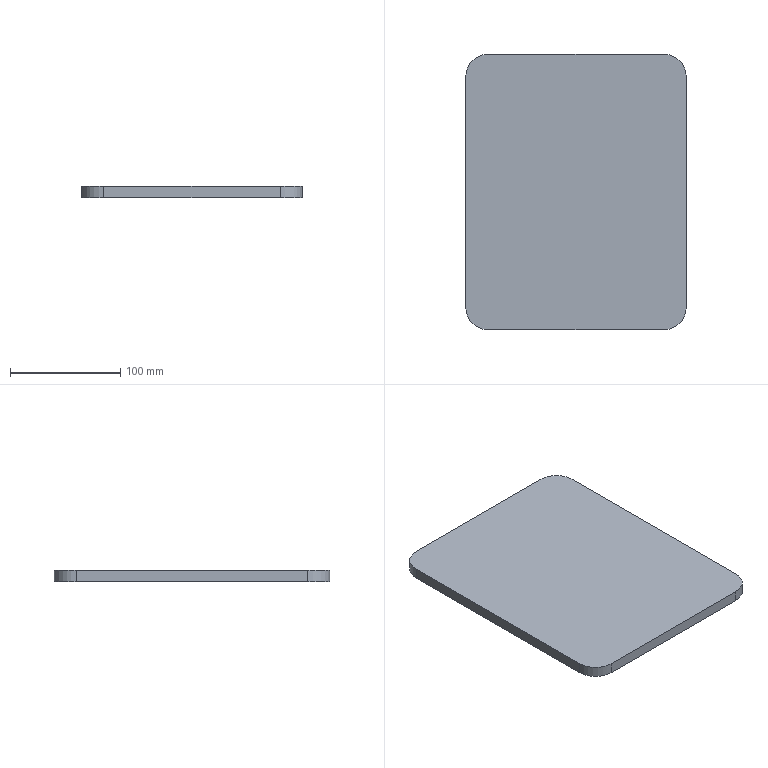Part | SolidWorks | features HoleWzd 2, Extrusion 1, Fillet 1 | 1 solid | 106 faces | box 200 x 250 x 10 mm | volume 494356 mm3 | cone 64 | cylinder 36 | plane 6 | commonest cylinder face diameters 5 x16 6.8 x16 40 x4